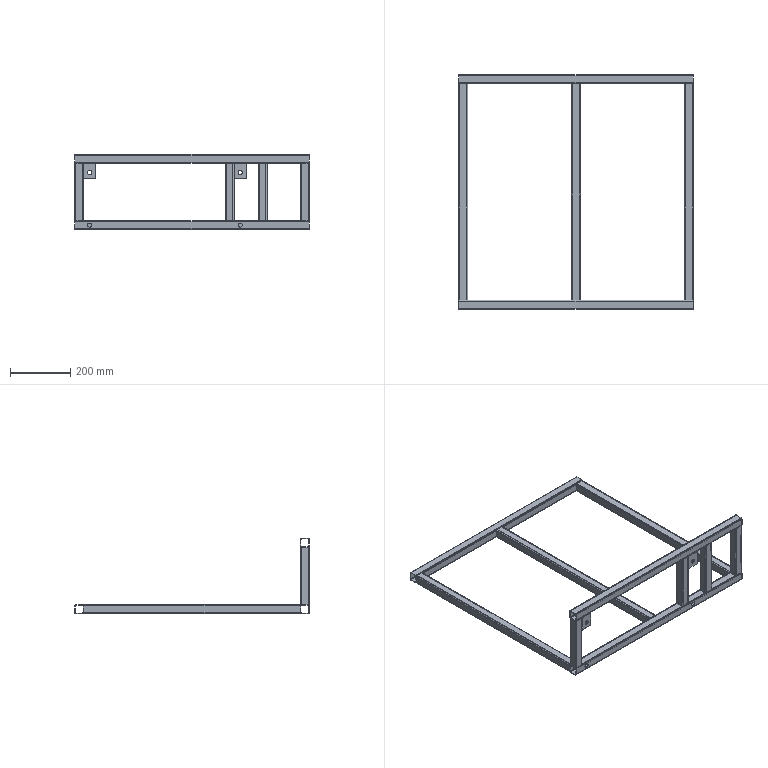Part | SolidWorks | features WeldCornerFeat 2, WeldMemberFeat 2, 3DProfileFeature 1, Cut 1, HoleWzd 1, MoveCopyBody 1, Split 1, WeldmentFeature 1 | 12 solids | 212 faces | box 780 x 780 x 250 mm | volume 1146296 mm3 | plane 116 | cylinder 96 | commonest cylinder face diameters 4 x40 8 x40 14 x12 2.667 x2 11 x2